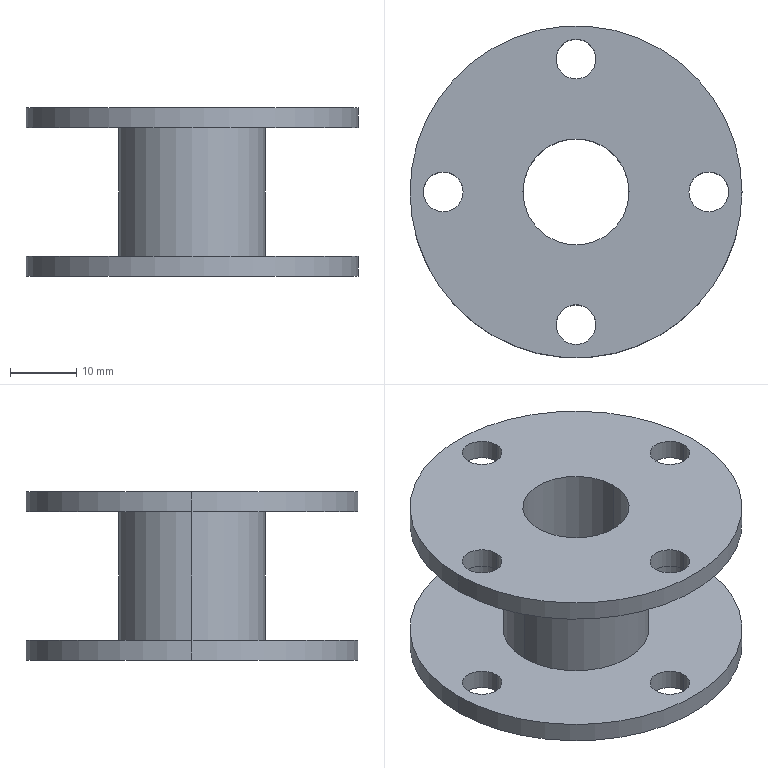Part | SolidWorks | features ExtruThin 1, ICE 1, MirrorPattern 1 | 1 solid | 28 faces | box 50 x 50 x 25.41 mm | volume 13372 mm3 | cylinder 24 | plane 4 | commonest cylinder face diameters 6 x16 50 x4 16 x2 22 x2
STEP:
#1=CARTESIAN_POINT('',(-23.,0.,-9.705));
#2=VERTEX_POINT('',#1);
#3=CARTESIAN_POINT('',(-17.,0.,-9.705));
#4=VERTEX_POINT('',#3);
#5=CARTESIAN_POINT('',(-20.,0.,-9.705));
#6=DIRECTION('',(0.,0.,1.));
#7=DIRECTION('',(1.,0.,0.));
#8=AXIS2_PLACEMENT_3D('',#5,#6,#7);
#9=CIRCLE('',#8,3.);
#10=EDGE_CURVE('',#2,#4,#9,.T.);
#11=ORIENTED_EDGE('',*,*,#10,.T.);
#12=CARTESIAN_POINT('',(-17.,0.,-12.705));
#13=VERTEX_POINT('',#12);
#14=CARTESIAN_POINT('',(-17.,0.,-9.705));
#15=DIRECTION('',(0.,0.,-1.));
#16=VECTOR('',#15,1000.);
#17=LINE('',#14,#16);
#18=EDGE_CURVE('',#4,#13,#17,.T.);
#19=ORIENTED_EDGE('',*,*,#18,.T.);
#20=CARTESIAN_POINT('',(-23.,0.,-12.705));
#21=VERTEX_POINT('',#20);
#22=CARTESIAN_POINT('',(-20.,0.,-12.705));
#23=DIRECTION('',(0.,0.,1.));
#24=DIRECTION('',(1.,0.,0.));
#25=AXIS2_PLACEMENT_3D('',#22,#23,#24);
#26=CIRCLE('',#25,3.);
#27=EDGE_CURVE('',#21,#13,#26,.T.);
#28=ORIENTED_EDGE('',*,*,#27,.F.);
#29=CARTESIAN_POINT('',(-23.,0.,-9.705));
#30=DIRECTION('',(0.,0.,-1.));
#31=VECTOR('',#30,1000.);
#32=LINE('',#29,#31);
#33=EDGE_CURVE('',#2,#21,#32,.T.);
#34=ORIENTED_EDGE('',*,*,#33,.F.);
#35=EDGE_LOOP('',(#11,#19,#28,#34));
#36=FACE_OUTER_BOUND('',#35,.T.);
#37=CARTESIAN_POINT('',(-20.,0.,-9.705));
#38=DIRECTION('',(0.,0.,-1.));
#39=DIRECTION('',(-1.,0.,0.));
#40=AXIS2_PLACEMENT_3D('',#37,#38,#39);
#41=CYLINDRICAL_SURFACE('',#40,3.);
#42=ADVANCED_FACE('',(#36),#41,.F.);
#43=CARTESIAN_POINT('',(-3.,-20.,-9.705));
#44=VERTEX_POINT('',#43);
#45=CARTESIAN_POINT('',(3.,-20.,-9.705));
#46=VERTEX_POINT('',#45);
#47=CARTESIAN_POINT('',(0.,-20.,-9.705));
#48=DIRECTION('',(0.,0.,1.));
#49=DIRECTION('',(1.,0.,0.));
#50=AXIS2_PLACEMENT_3D('',#47,#48,#49);
#51=CIRCLE('',#50,3.);
#52=EDGE_CURVE('',#44,#46,#51,.T.);
#53=ORIENTED_EDGE('',*,*,#52,.T.);
#54=CARTESIAN_POINT('',(3.,-20.,-12.705));
#55=VERTEX_POINT('',#54);
#56=CARTESIAN_POINT('',(3.,-20.,-9.705));
#57=DIRECTION('',(0.,0.,-1.));
#58=VECTOR('',#57,1000.);
#59=LINE('',#56,#58);
#60=EDGE_CURVE('',#46,#55,#59,.T.);
#61=ORIENTED_EDGE('',*,*,#60,.T.);
#62=CARTESIAN_POINT('',(-3.,-20.,-12.705));
#63=VERTEX_POINT('',#62);
#64=CARTESIAN_POINT('',(0.,-20.,-12.705));
#65=DIRECTION('',(0.,0.,1.));
#66=DIRECTION('',(1.,0.,0.));
#67=AXIS2_PLACEMENT_3D('',#64,#65,#66);
#68=CIRCLE('',#67,3.);
#69=EDGE_CURVE('',#63,#55,#68,.T.);
#70=ORIENTED_EDGE('',*,*,#69,.F.);
#71=CARTESIAN_POINT('',(-3.,-20.,-9.705));
#72=DIRECTION('',(0.,0.,-1.));
#73=VECTOR('',#72,1000.);
#74=LINE('',#71,#73);
#75=EDGE_CURVE('',#44,#63,#74,.T.);
#76=ORIENTED_EDGE('',*,*,#75,.F.);
#77=EDGE_LOOP('',(#53,#61,#70,#76));
#78=FACE_OUTER_BOUND('',#77,.T.);
#79=CARTESIAN_POINT('',(0.,-20.,-9.705));
#80=DIRECTION('',(0.,0.,-1.));
#81=DIRECTION('',(-1.,0.,0.));
#82=AXIS2_PLACEMENT_3D('',#79,#80,#81);
#83=CYLINDRICAL_SURFACE('',#82,3.);
#84=ADVANCED_FACE('',(#78),#83,.F.);
#85=CARTESIAN_POINT('',(17.,0.,-9.705));
#86=VERTEX_POINT('',#85);
#87=CARTESIAN_POINT('',(23.,0.,-9.705));
#88=VERTEX_POINT('',#87);
#89=CARTESIAN_POINT('',(20.,0.,-9.705));
#90=DIRECTION('',(0.,0.,1.));
#91=DIRECTION('',(1.,0.,0.));
#92=AXIS2_PLACEMENT_3D('',#89,#90,#91);
#93=CIRCLE('',#92,3.);
#94=EDGE_CURVE('',#86,#88,#93,.T.);
#95=ORIENTED_EDGE('',*,*,#94,.T.);
#96=CARTESIAN_POINT('',(23.,0.,-12.705));
#97=VERTEX_POINT('',#96);
#98=CARTESIAN_POINT('',(23.,0.,-9.705));
#99=DIRECTION('',(0.,0.,-1.));
#100=VECTOR('',#99,1000.);
#101=LINE('',#98,#100);
#102=EDGE_CURVE('',#88,#97,#101,.T.);
#103=ORIENTED_EDGE('',*,*,#102,.T.);
#104=CARTESIAN_POINT('',(17.,0.,-12.705));
#105=VERTEX_POINT('',#104);
#106=CARTESIAN_POINT('',(20.,0.,-12.705));
#107=DIRECTION('',(0.,0.,1.));
#108=DIRECTION('',(1.,0.,0.));
#109=AXIS2_PLACEMENT_3D('',#106,#107,#108);
#110=CIRCLE('',#109,3.);
#111=EDGE_CURVE('',#105,#97,#110,.T.);
#112=ORIENTED_EDGE('',*,*,#111,.F.);
#113=CARTESIAN_POINT('',(17.,0.,-9.705));
#114=DIRECTION('',(0.,0.,-1.));
#115=VECTOR('',#114,1000.);
#116=LINE('',#113,#115);
#117=EDGE_CURVE('',#86,#105,#116,.T.);
#118=ORIENTED_EDGE('',*,*,#117,.F.);
#119=EDGE_LOOP('',(#95,#103,#112,#118));
#120=FACE_OUTER_BOUND('',#119,.T.);
#121=CARTESIAN_POINT('',(20.,0.,-9.705));
#122=DIRECTION('',(0.,0.,-1.));
#123=DIRECTION('',(-1.,0.,0.));
#124=AXIS2_PLACEMENT_3D('',#121,#122,#123);
#125=CYLINDRICAL_SURFACE('',#124,3.);
#126=ADVANCED_FACE('',(#120),#125,.F.);
#127=CARTESIAN_POINT('',(-3.,20.,-9.705));
#128=VERTEX_POINT('',#127);
#129=CARTESIAN_POINT('',(3.,20.,-9.705));
#130=VERTEX_POINT('',#129);
#131=CARTESIAN_POINT('',(0.,20.,-9.705));
#132=DIRECTION('',(0.,0.,1.));
#133=DIRECTION('',(1.,0.,0.));
#134=AXIS2_PLACEMENT_3D('',#131,#132,#133);
#135=CIRCLE('',#134,3.);
#136=EDGE_CURVE('',#128,#130,#135,.T.);
#137=ORIENTED_EDGE('',*,*,#136,.T.);
#138=CARTESIAN_POINT('',(3.,20.,-12.705));
#139=VERTEX_POINT('',#138);
#140=CARTESIAN_POINT('',(3.,20.,-9.705));
#141=DIRECTION('',(0.,0.,-1.));
#142=VECTOR('',#141,1000.);
#143=LINE('',#140,#142);
#144=EDGE_CURVE('',#130,#139,#143,.T.);
#145=ORIENTED_EDGE('',*,*,#144,.T.);
#146=CARTESIAN_POINT('',(-3.,20.,-12.705));
#147=VERTEX_POINT('',#146);
#148=CARTESIAN_POINT('',(0.,20.,-12.705));
#149=DIRECTION('',(0.,0.,1.));
#150=DIRECTION('',(1.,0.,0.));
#151=AXIS2_PLACEMENT_3D('',#148,#149,#150);
#152=CIRCLE('',#151,3.);
#153=EDGE_CURVE('',#147,#139,#152,.T.);
#154=ORIENTED_EDGE('',*,*,#153,.F.);
#155=CARTESIAN_POINT('',(-3.,20.,-9.705));
#156=DIRECTION('',(0.,0.,-1.));
#157=VECTOR('',#156,1000.);
#158=LINE('',#155,#157);
#159=EDGE_CURVE('',#128,#147,#158,.T.);
#160=ORIENTED_EDGE('',*,*,#159,.F.);
#161=EDGE_LOOP('',(#137,#145,#154,#160));
#162=FACE_OUTER_BOUND('',#161,.T.);
#163=CARTESIAN_POINT('',(0.,20.,-9.705));
#164=DIRECTION('',(0.,0.,-1.));
#165=DIRECTION('',(-1.,0.,0.));
#166=AXIS2_PLACEMENT_3D('',#163,#164,#165);
#167=CYLINDRICAL_SURFACE('',#166,3.);
#168=ADVANCED_FACE('',(#162),#167,.F.);
#169=CARTESIAN_POINT('',(25.,0.,-9.705));
#170=VERTEX_POINT('',#169);
#171=CARTESIAN_POINT('',(-25.,0.,-9.705));
#172=VERTEX_POINT('',#171);
#173=CARTESIAN_POINT('',(0.,0.,-9.705));
#174=DIRECTION('',(0.,0.,1.));
#175=DIRECTION('',(1.,0.,0.));
#176=AXIS2_PLACEMENT_3D('',#173,#174,#175);
#177=CIRCLE('',#176,25.);
#178=EDGE_CURVE('',#170,#172,#177,.T.);
#179=ORIENTED_EDGE('',*,*,#178,.F.);
#180=CARTESIAN_POINT('',(25.,0.,-12.705));
#181=VERTEX_POINT('',#180);
#182=CARTESIAN_POINT('',(25.,0.,-9.705));
#183=DIRECTION('',(0.,0.,-1.));
#184=VECTOR('',#183,1000.);
#185=LINE('',#182,#184);
#186=EDGE_CURVE('',#170,#181,#185,.T.);
#187=ORIENTED_EDGE('',*,*,#186,.T.);
#188=CARTESIAN_POINT('',(-25.,0.,-12.705));
#189=VERTEX_POINT('',#188);
#190=CARTESIAN_POINT('',(0.,0.,-12.705));
#191=DIRECTION('',(0.,0.,1.));
#192=DIRECTION('',(1.,0.,0.));
#193=AXIS2_PLACEMENT_3D('',#190,#191,#192);
#194=CIRCLE('',#193,25.);
#195=EDGE_CURVE('',#181,#189,#194,.T.);
#196=ORIENTED_EDGE('',*,*,#195,.T.);
#197=CARTESIAN_POINT('',(-25.,0.,-9.705));
#198=DIRECTION('',(0.,0.,-1.));
#199=VECTOR('',#198,1000.);
#200=LINE('',#197,#199);
#201=EDGE_CURVE('',#172,#189,#200,.T.);
#202=ORIENTED_EDGE('',*,*,#201,.F.);
#203=EDGE_LOOP('',(#179,#187,#196,#202));
#204=FACE_OUTER_BOUND('',#203,.T.);
#205=CARTESIAN_POINT('',(0.,0.,-9.705));
#206=DIRECTION('',(0.,0.,-1.));
#207=DIRECTION('',(-1.,0.,0.));
#208=AXIS2_PLACEMENT_3D('',#205,#206,#207);
#209=CYLINDRICAL_SURFACE('',#208,25.);
#210=ADVANCED_FACE('',(#204),#209,.T.);
#211=CARTESIAN_POINT('',(-23.,0.,9.705));
#212=VERTEX_POINT('',#211);
#213=CARTESIAN_POINT('',(-17.,0.,9.705));
#214=VERTEX_POINT('',#213);
#215=CARTESIAN_POINT('',(-20.,0.,9.705));
#216=DIRECTION('',(0.,0.,1.));
#217=DIRECTION('',(1.,0.,0.));
#218=AXIS2_PLACEMENT_3D('',#215,#216,#217);
#219=CIRCLE('',#218,3.);
#220=EDGE_CURVE('',#212,#214,#219,.T.);
#221=ORIENTED_EDGE('',*,*,#220,.F.);
#222=CARTESIAN_POINT('',(-23.,0.,12.705));
#223=VERTEX_POINT('',#222);
#224=CARTESIAN_POINT('',(-23.,0.,9.705));
#225=DIRECTION('',(0.,0.,1.));
#226=VECTOR('',#225,1000.);
#227=LINE('',#224,#226);
#228=EDGE_CURVE('',#212,#223,#227,.T.);
#229=ORIENTED_EDGE('',*,*,#228,.T.);
#230=CARTESIAN_POINT('',(-17.,0.,12.705));
#231=VERTEX_POINT('',#230);
#232=CARTESIAN_POINT('',(-20.,0.,12.705));
#233=DIRECTION('',(0.,0.,1.));
#234=DIRECTION('',(1.,0.,0.));
#235=AXIS2_PLACEMENT_3D('',#232,#233,#234);
#236=CIRCLE('',#235,3.);
#237=EDGE_CURVE('',#223,#231,#236,.T.);
#238=ORIENTED_EDGE('',*,*,#237,.T.);
#239=CARTESIAN_POINT('',(-17.,0.,9.705));
#240=DIRECTION('',(0.,0.,1.));
#241=VECTOR('',#240,1000.);
#242=LINE('',#239,#241);
#243=EDGE_CURVE('',#214,#231,#242,.T.);
#244=ORIENTED_EDGE('',*,*,#243,.F.);
#245=EDGE_LOOP('',(#221,#229,#238,#244));
#246=FACE_OUTER_BOUND('',#245,.T.);
#247=CARTESIAN_POINT('',(-20.,0.,9.705));
#248=DIRECTION('',(0.,0.,1.));
#249=DIRECTION('',(1.,0.,0.));
#250=AXIS2_PLACEMENT_3D('',#247,#248,#249);
#251=CYLINDRICAL_SURFACE('',#250,3.);
#252=ADVANCED_FACE('',(#246),#251,.F.);
#253=CARTESIAN_POINT('',(-3.,-20.,9.705));
#254=VERTEX_POINT('',#253);
#255=CARTESIAN_POINT('',(3.,-20.,9.705));
#256=VERTEX_POINT('',#255);
#257=CARTESIAN_POINT('',(0.,-20.,9.705));
#258=DIRECTION('',(0.,0.,1.));
#259=DIRECTION('',(1.,0.,0.));
#260=AXIS2_PLACEMENT_3D('',#257,#258,#259);
#261=CIRCLE('',#260,3.);
#262=EDGE_CURVE('',#254,#256,#261,.T.);
#263=ORIENTED_EDGE('',*,*,#262,.F.);
#264=CARTESIAN_POINT('',(-3.,-20.,12.705));
#265=VERTEX_POINT('',#264);
#266=CARTESIAN_POINT('',(-3.,-20.,9.705));
#267=DIRECTION('',(0.,0.,1.));
#268=VECTOR('',#267,1000.);
#269=LINE('',#266,#268);
#270=EDGE_CURVE('',#254,#265,#269,.T.);
#271=ORIENTED_EDGE('',*,*,#270,.T.);
#272=CARTESIAN_POINT('',(3.,-20.,12.705));
#273=VERTEX_POINT('',#272);
#274=CARTESIAN_POINT('',(0.,-20.,12.705));
#275=DIRECTION('',(0.,0.,1.));
#276=DIRECTION('',(1.,0.,0.));
#277=AXIS2_PLACEMENT_3D('',#274,#275,#276);
#278=CIRCLE('',#277,3.);
#279=EDGE_CURVE('',#265,#273,#278,.T.);
#280=ORIENTED_EDGE('',*,*,#279,.T.);
#281=CARTESIAN_POINT('',(3.,-20.,9.705));
#282=DIRECTION('',(0.,0.,1.));
#283=VECTOR('',#282,1000.);
#284=LINE('',#281,#283);
#285=EDGE_CURVE('',#256,#273,#284,.T.);
#286=ORIENTED_EDGE('',*,*,#285,.F.);
#287=EDGE_LOOP('',(#263,#271,#280,#286));
#288=FACE_OUTER_BOUND('',#287,.T.);
#289=CARTESIAN_POINT('',(0.,-20.,9.705));
#290=DIRECTION('',(0.,0.,1.));
#291=DIRECTION('',(1.,0.,0.));
#292=AXIS2_PLACEMENT_3D('',#289,#290,#291);
#293=CYLINDRICAL_SURFACE('',#292,3.);
#294=ADVANCED_FACE('',(#288),#293,.F.);
#295=CARTESIAN_POINT('',(17.,0.,9.705));
#296=VERTEX_POINT('',#295);
#297=CARTESIAN_POINT('',(23.,0.,9.705));
#298=VERTEX_POINT('',#297);
#299=CARTESIAN_POINT('',(20.,0.,9.705));
#300=DIRECTION('',(0.,0.,1.));
#301=DIRECTION('',(1.,0.,0.));
#302=AXIS2_PLACEMENT_3D('',#299,#300,#301);
#303=CIRCLE('',#302,3.);
#304=EDGE_CURVE('',#296,#298,#303,.T.);
#305=ORIENTED_EDGE('',*,*,#304,.F.);
#306=CARTESIAN_POINT('',(17.,0.,12.705));
#307=VERTEX_POINT('',#306);
#308=CARTESIAN_POINT('',(17.,0.,9.705));
#309=DIRECTION('',(0.,0.,1.));
#310=VECTOR('',#309,1000.);
#311=LINE('',#308,#310);
#312=EDGE_CURVE('',#296,#307,#311,.T.);
#313=ORIENTED_EDGE('',*,*,#312,.T.);
#314=CARTESIAN_POINT('',(23.,0.,12.705));
#315=VERTEX_POINT('',#314);
#316=CARTESIAN_POINT('',(20.,0.,12.705));
#317=DIRECTION('',(0.,0.,1.));
#318=DIRECTION('',(1.,0.,0.));
#319=AXIS2_PLACEMENT_3D('',#316,#317,#318);
#320=CIRCLE('',#319,3.);
#321=EDGE_CURVE('',#307,#315,#320,.T.);
#322=ORIENTED_EDGE('',*,*,#321,.T.);
#323=CARTESIAN_POINT('',(23.,0.,9.705));
#324=DIRECTION('',(0.,0.,1.));
#325=VECTOR('',#324,1000.);
#326=LINE('',#323,#325);
#327=EDGE_CURVE('',#298,#315,#326,.T.);
#328=ORIENTED_EDGE('',*,*,#327,.F.);
#329=EDGE_LOOP('',(#305,#313,#322,#328));
#330=FACE_OUTER_BOUND('',#329,.T.);
#331=CARTESIAN_POINT('',(20.,0.,9.705));
#332=DIRECTION('',(0.,0.,1.));
#333=DIRECTION('',(1.,0.,0.));
#334=AXIS2_PLACEMENT_3D('',#331,#332,#333);
#335=CYLINDRICAL_SURFACE('',#334,3.);
#336=ADVANCED_FACE('',(#330),#335,.F.);
#337=CARTESIAN_POINT('',(-3.,20.,9.705));
#338=VERTEX_POINT('',#337);
#339=CARTESIAN_POINT('',(3.,20.,9.705));
#340=VERTEX_POINT('',#339);
#341=CARTESIAN_POINT('',(0.,20.,9.705));
#342=DIRECTION('',(0.,0.,1.));
#343=DIRECTION('',(1.,0.,0.));
#344=AXIS2_PLACEMENT_3D('',#341,#342,#343);
#345=CIRCLE('',#344,3.);
#346=EDGE_CURVE('',#338,#340,#345,.T.);
#347=ORIENTED_EDGE('',*,*,#346,.F.);
#348=CARTESIAN_POINT('',(-3.,20.,12.705));
#349=VERTEX_POINT('',#348);
#350=CARTESIAN_POINT('',(-3.,20.,9.705));
#351=DIRECTION('',(0.,0.,1.));
#352=VECTOR('',#351,1000.);
#353=LINE('',#350,#352);
#354=EDGE_CURVE('',#338,#349,#353,.T.);
#355=ORIENTED_EDGE('',*,*,#354,.T.);
#356=CARTESIAN_POINT('',(3.,20.,12.705));
#357=VERTEX_POINT('',#356);
#358=CARTESIAN_POINT('',(0.,20.,12.705));
#359=DIRECTION('',(0.,0.,1.));
#360=DIRECTION('',(1.,0.,0.));
#361=AXIS2_PLACEMENT_3D('',#358,#359,#360);
#362=CIRCLE('',#361,3.);
#363=EDGE_CURVE('',#349,#357,#362,.T.);
#364=ORIENTED_EDGE('',*,*,#363,.T.);
#365=CARTESIAN_POINT('',(3.,20.,9.705));
#366=DIRECTION('',(0.,0.,1.));
#367=VECTOR('',#366,1000.);
#368=LINE('',#365,#367);
#369=EDGE_CURVE('',#340,#357,#368,.T.);
#370=ORIENTED_EDGE('',*,*,#369,.F.);
#371=EDGE_LOOP('',(#347,#355,#364,#370));
#372=FACE_OUTER_BOUND('',#371,.T.);
#373=CARTESIAN_POINT('',(0.,20.,9.705));
#374=DIRECTION('',(0.,0.,1.));
#375=DIRECTION('',(1.,0.,0.));
#376=AXIS2_PLACEMENT_3D('',#373,#374,#375);
#377=CYLINDRICAL_SURFACE('',#376,3.);
#378=ADVANCED_FACE('',(#372),#377,.F.);
#379=CARTESIAN_POINT('',(25.,0.,9.705));
#380=VERTEX_POINT('',#379);
#381=CARTESIAN_POINT('',(-25.,0.,9.705));
#382=VERTEX_POINT('',#381);
#383=CARTESIAN_POINT('',(0.,0.,9.705));
#384=DIRECTION('',(0.,0.,1.));
#385=DIRECTION('',(1.,0.,0.));
#386=AXIS2_PLACEMENT_3D('',#383,#384,#385);
#387=CIRCLE('',#386,25.);
#388=EDGE_CURVE('',#380,#382,#387,.T.);
#389=ORIENTED_EDGE('',*,*,#388,.T.);
#390=CARTESIAN_POINT('',(-25.,0.,12.705));
#391=VERTEX_POINT('',#390);
#392=CARTESIAN_POINT('',(-25.,0.,9.705));
#393=DIRECTION('',(0.,0.,1.));
#394=VECTOR('',#393,1000.);
#395=LINE('',#392,#394);
#396=EDGE_CURVE('',#382,#391,#395,.T.);
#397=ORIENTED_EDGE('',*,*,#396,.T.);
#398=CARTESIAN_POINT('',(25.,0.,12.705));
#399=VERTEX_POINT('',#398);
#400=CARTESIAN_POINT('',(0.,0.,12.705));
#401=DIRECTION('',(0.,0.,1.));
#402=DIRECTION('',(1.,0.,0.));
#403=AXIS2_PLACEMENT_3D('',#400,#401,#402);
#404=CIRCLE('',#403,25.);
#405=EDGE_CURVE('',#399,#391,#404,.T.);
#406=ORIENTED_EDGE('',*,*,#405,.F.);
#407=CARTESIAN_POINT('',(25.,0.,9.705));
#408=DIRECTION('',(0.,0.,1.));
#409=VECTOR('',#408,1000.);
#410=LINE('',#407,#409);
#411=EDGE_CURVE('',#380,#399,#410,.T.);
#412=ORIENTED_EDGE('',*,*,#411,.F.);
#413=EDGE_LOOP('',(#389,#397,#406,#412));
#414=FACE_OUTER_BOUND('',#413,.T.);
#415=CARTESIAN_POINT('',(0.,0.,9.705));
#416=DIRECTION('',(0.,0.,1.));
#417=DIRECTION('',(1.,0.,0.));
#418=AXIS2_PLACEMENT_3D('',#415,#416,#417);
#419=CYLINDRICAL_SURFACE('',#418,25.);
#420=ADVANCED_FACE('',(#414),#419,.T.);
#421=CARTESIAN_POINT('',(-8.,0.,12.705));
#422=VERTEX_POINT('',#421);
#423=CARTESIAN_POINT('',(8.,0.,12.705));
#424=VERTEX_POINT('',#423);
#425=CARTESIAN_POINT('',(0.,0.,12.705));
#426=DIRECTION('',(0.,0.,1.));
#427=DIRECTION('',(1.,0.,0.));
#428=AXIS2_PLACEMENT_3D('',#425,#426,#427);
#429=CIRCLE('',#428,8.);
#430=EDGE_CURVE('',#422,#424,#429,.T.);
#431=ORIENTED_EDGE('',*,*,#430,.T.);
#432=CARTESIAN_POINT('',(8.,0.,-12.705));
#433=VERTEX_POINT('',#432);
#434=CARTESIAN_POINT('',(8.,0.,12.705));
#435=DIRECTION('',(0.,0.,-1.));
#436=VECTOR('',#435,1000.);
#437=LINE('',#434,#436);
#438=EDGE_CURVE('',#424,#433,#437,.T.);
#439=ORIENTED_EDGE('',*,*,#438,.T.);
#440=CARTESIAN_POINT('',(-8.,0.,-12.705));
#441=VERTEX_POINT('',#440);
#442=CARTESIAN_POINT('',(0.,0.,-12.705));
#443=DIRECTION('',(0.,0.,1.));
#444=DIRECTION('',(1.,0.,0.));
#445=AXIS2_PLACEMENT_3D('',#442,#443,#444);
#446=CIRCLE('',#445,8.);
#447=EDGE_CURVE('',#441,#433,#446,.T.);
#448=ORIENTED_EDGE('',*,*,#447,.F.);
#449=CARTESIAN_POINT('',(-8.,0.,12.705));
#450=DIRECTION('',(0.,0.,-1.));
#451=VECTOR('',#450,1000.);
#452=LINE('',#449,#451);
#453=EDGE_CURVE('',#422,#441,#452,.T.);
#454=ORIENTED_EDGE('',*,*,#453,.F.);
#455=EDGE_LOOP('',(#431,#439,#448,#454));
#456=FACE_OUTER_BOUND('',#455,.T.);
#457=CARTESIAN_POINT('',(0.,0.,12.705));
#458=DIRECTION('',(0.,0.,-1.));
#459=DIRECTION('',(-1.,0.,0.));
#460=AXIS2_PLACEMENT_3D('',#457,#458,#459);
#461=CYLINDRICAL_SURFACE('',#460,8.);
#462=ADVANCED_FACE('',(#456),#461,.F.);
#463=CARTESIAN_POINT('',(11.,0.,9.705));
#464=VERTEX_POINT('',#463);
#465=CARTESIAN_POINT('',(-11.,0.,9.705));
#466=VERTEX_POINT('',#465);
#467=CARTESIAN_POINT('',(0.,0.,9.705));
#468=DIRECTION('',(0.,0.,1.));
#469=DIRECTION('',(1.,0.,0.));
#470=AXIS2_PLACEMENT_3D('',#467,#468,#469);
#471=CIRCLE('',#470,11.);
#472=EDGE_CURVE('',#464,#466,#471,.T.);
#473=ORIENTED_EDGE('',*,*,#472,.F.);
#474=CARTESIAN_POINT('',(11.,0.,-9.705));
#475=VERTEX_POINT('',#474);
#476=CARTESIAN_POINT('',(11.,0.,12.705));
#477=DIRECTION('',(0.,0.,-1.));
#478=VECTOR('',#477,1000.);
#479=LINE('',#476,#478);
#480=EDGE_CURVE('',#464,#475,#479,.T.);
#481=ORIENTED_EDGE('',*,*,#480,.T.);
#482=CARTESIAN_POINT('',(-11.,0.,-9.705));
#483=VERTEX_POINT('',#482);
#484=CARTESIAN_POINT('',(0.,0.,-9.705));
#485=DIRECTION('',(0.,0.,-1.));
#486=DIRECTION('',(-1.,0.,0.));
#487=AXIS2_PLACEMENT_3D('',#484,#485,#486);
#488=CIRCLE('',#487,11.);
#489=EDGE_CURVE('',#483,#475,#488,.T.);
#490=ORIENTED_EDGE('',*,*,#489,.F.);
#491=CARTESIAN_POINT('',(-11.,0.,12.705));
#492=DIRECTION('',(0.,0.,-1.));
#493=VECTOR('',#492,1000.);
#494=LINE('',#491,#493);
#495=EDGE_CURVE('',#466,#483,#494,.T.);
#496=ORIENTED_EDGE('',*,*,#495,.F.);
#497=EDGE_LOOP('',(#473,#481,#490,#496));
#498=FACE_OUTER_BOUND('',#497,.T.);
#499=CARTESIAN_POINT('',(0.,0.,12.705));
#500=DIRECTION('',(0.,0.,-1.));
#501=DIRECTION('',(-1.,0.,0.));
#502=AXIS2_PLACEMENT_3D('',#499,#500,#501);
#503=CYLINDRICAL_SURFACE('',#502,11.);
#504=ADVANCED_FACE('',(#498),#503,.T.);
#505=ORIENTED_EDGE('',*,*,#480,.F.);
#506=CARTESIAN_POINT('',(0.,0.,9.705));
#507=DIRECTION('',(0.,0.,1.));
#508=DIRECTION('',(1.,0.,0.));
#509=AXIS2_PLACEMENT_3D('',#506,#507,#508);
#510=CIRCLE('',#509,11.);
#511=EDGE_CURVE('',#466,#464,#510,.T.);
#512=ORIENTED_EDGE('',*,*,#511,.F.);
#513=ORIENTED_EDGE('',*,*,#495,.T.);
#514=CARTESIAN_POINT('',(0.,0.,-9.705));
#515=DIRECTION('',(0.,0.,-1.));
#516=DIRECTION('',(-1.,0.,0.));
#517=AXIS2_PLACEMENT_3D('',#514,#515,#516);
#518=CIRCLE('',#517,11.);
#519=EDGE_CURVE('',#475,#483,#518,.T.);
#520=ORIENTED_EDGE('',*,*,#519,.F.);
#521=EDGE_LOOP('',(#505,#512,#513,#520));
#522=FACE_OUTER_BOUND('',#521,.T.);
#523=CARTESIAN_POINT('',(0.,0.,12.705));
#524=DIRECTION('',(0.,0.,-1.));
#525=DIRECTION('',(-1.,0.,0.));
#526=AXIS2_PLACEMENT_3D('',#523,#524,#525);
#527=CYLINDRICAL_SURFACE('',#526,11.);
#528=ADVANCED_FACE('',(#522),#527,.T.);
#529=ORIENTED_EDGE('',*,*,#430,.F.);
#530=CARTESIAN_POINT('',(0.,0.,12.705));
#531=DIRECTION('',(0.,0.,1.));
#532=DIRECTION('',(1.,0.,0.));
#533=AXIS2_PLACEMENT_3D('',#530,#531,#532);
#534=CIRCLE('',#533,8.);
#535=EDGE_CURVE('',#424,#422,#534,.T.);
#536=ORIENTED_EDGE('',*,*,#535,.F.);
#537=EDGE_LOOP('',(#529,#536));
#538=FACE_BOUND('',#537,.T.);
#539=ORIENTED_EDGE('',*,*,#405,.T.);
#540=CARTESIAN_POINT('',(0.,0.,12.705));
#541=DIRECTION('',(0.,0.,1.));
#542=DIRECTION('',(1.,0.,0.));
#543=AXIS2_PLACEMENT_3D('',#540,#541,#542);
#544=CIRCLE('',#543,25.);
#545=EDGE_CURVE('',#391,#399,#544,.T.);
#546=ORIENTED_EDGE('',*,*,#545,.T.);
#547=EDGE_LOOP('',(#539,#546));
#548=FACE_OUTER_BOUND('',#547,.T.);
#549=CARTESIAN_POINT('',(0.,20.,12.705));
#550=DIRECTION('',(0.,0.,1.));
#551=DIRECTION('',(1.,0.,0.));
#552=AXIS2_PLACEMENT_3D('',#549,#550,#551);
#553=CIRCLE('',#552,3.);
#554=EDGE_CURVE('',#357,#349,#553,.T.);
#555=ORIENTED_EDGE('',*,*,#554,.F.);
#556=ORIENTED_EDGE('',*,*,#363,.F.);
#557=EDGE_LOOP('',(#555,#556));
#558=FACE_BOUND('',#557,.T.);
#559=CARTESIAN_POINT('',(20.,0.,12.705));
#560=DIRECTION('',(0.,0.,1.));
#561=DIRECTION('',(1.,0.,0.));
#562=AXIS2_PLACEMENT_3D('',#559,#560,#561);
#563=CIRCLE('',#562,3.);
#564=EDGE_CURVE('',#315,#307,#563,.T.);
#565=ORIENTED_EDGE('',*,*,#564,.F.);
#566=ORIENTED_EDGE('',*,*,#321,.F.);
#567=EDGE_LOOP('',(#565,#566));
#568=FACE_BOUND('',#567,.T.);
#569=CARTESIAN_POINT('',(0.,-20.,12.705));
#570=DIRECTION('',(0.,0.,1.));
#571=DIRECTION('',(1.,0.,0.));
#572=AXIS2_PLACEMENT_3D('',#569,#570,#571);
#573=CIRCLE('',#572,3.);
#574=EDGE_CURVE('',#273,#265,#573,.T.);
#575=ORIENTED_EDGE('',*,*,#574,.F.);
#576=ORIENTED_EDGE('',*,*,#279,.F.);
#577=EDGE_LOOP('',(#575,#576));
#578=FACE_BOUND('',#577,.T.);
#579=CARTESIAN_POINT('',(-20.,0.,12.705));
#580=DIRECTION('',(0.,0.,1.));
#581=DIRECTION('',(1.,0.,0.));
#582=AXIS2_PLACEMENT_3D('',#579,#580,#581);
#583=CIRCLE('',#582,3.);
#584=EDGE_CURVE('',#231,#223,#583,.T.);
#585=ORIENTED_EDGE('',*,*,#584,.F.);
#586=ORIENTED_EDGE('',*,*,#237,.F.);
#587=EDGE_LOOP('',(#585,#586));
#588=FACE_BOUND('',#587,.T.);
#589=CARTESIAN_POINT('',(0.,0.,12.705));
#590=DIRECTION('',(0.,0.,1.));
#591=DIRECTION('',(1.,0.,0.));
#592=AXIS2_PLACEMENT_3D('',#589,#590,#591);
#593=PLANE('',#592);
#594=ADVANCED_FACE('',(#538,#548,#558,#568,#578,#588),#593,.T.);
#595=ORIENTED_EDGE('',*,*,#447,.T.);
#596=CARTESIAN_POINT('',(0.,0.,-12.705));
#597=DIRECTION('',(0.,0.,1.));
#598=DIRECTION('',(1.,0.,0.));
#599=AXIS2_PLACEMENT_3D('',#596,#597,#598);
#600=CIRCLE('',#599,8.);
#601=EDGE_CURVE('',#433,#441,#600,.T.);
#602=ORIENTED_EDGE('',*,*,#601,.T.);
#603=EDGE_LOOP('',(#595,#602));
#604=FACE_BOUND('',#603,.T.);
#605=ORIENTED_EDGE('',*,*,#27,.T.);
#606=CARTESIAN_POINT('',(-20.,0.,-12.705));
#607=DIRECTION('',(0.,0.,1.));
#608=DIRECTION('',(1.,0.,0.));
#609=AXIS2_PLACEMENT_3D('',#606,#607,#608);
#610=CIRCLE('',#609,3.);
#611=EDGE_CURVE('',#13,#21,#610,.T.);
#612=ORIENTED_EDGE('',*,*,#611,.T.);
#613=EDGE_LOOP('',(#605,#612));
#614=FACE_BOUND('',#613,.T.);
#615=ORIENTED_EDGE('',*,*,#111,.T.);
#616=CARTESIAN_POINT('',(20.,0.,-12.705));
#617=DIRECTION('',(0.,0.,1.));
#618=DIRECTION('',(1.,0.,0.));
#619=AXIS2_PLACEMENT_3D('',#616,#617,#618);
#620=CIRCLE('',#619,3.);
#621=EDGE_CURVE('',#97,#105,#620,.T.);
#622=ORIENTED_EDGE('',*,*,#621,.T.);
#623=EDGE_LOOP('',(#615,#622));
#624=FACE_BOUND('',#623,.T.);
#625=CARTESIAN_POINT('',(0.,0.,-12.705));
#626=DIRECTION('',(0.,0.,1.));
#627=DIRECTION('',(1.,0.,0.));
#628=AXIS2_PLACEMENT_3D('',#625,#626,#627);
#629=CIRCLE('',#628,25.);
#630=EDGE_CURVE('',#189,#181,#629,.T.);
#631=ORIENTED_EDGE('',*,*,#630,.F.);
#632=ORIENTED_EDGE('',*,*,#195,.F.);
#633=EDGE_LOOP('',(#631,#632));
#634=FACE_OUTER_BOUND('',#633,.T.);
#635=ORIENTED_EDGE('',*,*,#153,.T.);
#636=CARTESIAN_POINT('',(0.,20.,-12.705));
#637=DIRECTION('',(0.,0.,1.));
#638=DIRECTION('',(1.,0.,0.));
#639=AXIS2_PLACEMENT_3D('',#636,#637,#638);
#640=CIRCLE('',#639,3.);
#641=EDGE_CURVE('',#139,#147,#640,.T.);
#642=ORIENTED_EDGE('',*,*,#641,.T.);
#643=EDGE_LOOP('',(#635,#642));
#644=FACE_BOUND('',#643,.T.);
#645=ORIENTED_EDGE('',*,*,#69,.T.);
#646=CARTESIAN_POINT('',(0.,-20.,-12.705));
#647=DIRECTION('',(0.,0.,1.));
#648=DIRECTION('',(1.,0.,0.));
#649=AXIS2_PLACEMENT_3D('',#646,#647,#648);
#650=CIRCLE('',#649,3.);
#651=EDGE_CURVE('',#55,#63,#650,.T.);
#652=ORIENTED_EDGE('',*,*,#651,.T.);
#653=EDGE_LOOP('',(#645,#652));
#654=FACE_BOUND('',#653,.T.);
#655=CARTESIAN_POINT('',(0.,0.,-12.705));
#656=DIRECTION('',(0.,0.,1.));
#657=DIRECTION('',(1.,0.,0.));
#658=AXIS2_PLACEMENT_3D('',#655,#656,#657);
#659=PLANE('',#658);
#660=ADVANCED_FACE('',(#604,#614,#624,#634,#644,#654),#659,.F.);
#661=ORIENTED_EDGE('',*,*,#438,.F.);
#662=ORIENTED_EDGE('',*,*,#535,.T.);
#663=ORIENTED_EDGE('',*,*,#453,.T.);
#664=ORIENTED_EDGE('',*,*,#601,.F.);
#665=EDGE_LOOP('',(#661,#662,#663,#664));
#666=FACE_OUTER_BOUND('',#665,.T.);
#667=CARTESIAN_POINT('',(0.,0.,12.705));
#668=DIRECTION('',(0.,0.,-1.));
#669=DIRECTION('',(-1.,0.,0.));
#670=AXIS2_PLACEMENT_3D('',#667,#668,#669);
#671=CYLINDRICAL_SURFACE('',#670,8.);
#672=ADVANCED_FACE('',(#666),#671,.F.);
#673=ORIENTED_EDGE('',*,*,#388,.F.);
#674=CARTESIAN_POINT('',(0.,0.,9.705));
#675=DIRECTION('',(0.,0.,1.));
#676=DIRECTION('',(1.,0.,0.));
#677=AXIS2_PLACEMENT_3D('',#674,#675,#676);
#678=CIRCLE('',#677,25.);
#679=EDGE_CURVE('',#382,#380,#678,.T.);
#680=ORIENTED_EDGE('',*,*,#679,.F.);
#681=EDGE_LOOP('',(#673,#680));
#682=FACE_OUTER_BOUND('',#681,.T.);
#683=CARTESIAN_POINT('',(0.,20.,9.705));
#684=DIRECTION('',(0.,0.,1.));
#685=DIRECTION('',(1.,0.,0.));
#686=AXIS2_PLACEMENT_3D('',#683,#684,#685);
#687=CIRCLE('',#686,3.);
#688=EDGE_CURVE('',#340,#338,#687,.T.);
#689=ORIENTED_EDGE('',*,*,#688,.T.);
#690=ORIENTED_EDGE('',*,*,#346,.T.);
#691=EDGE_LOOP('',(#689,#690));
#692=FACE_BOUND('',#691,.T.);
#693=CARTESIAN_POINT('',(20.,0.,9.705));
#694=DIRECTION('',(0.,0.,1.));
#695=DIRECTION('',(1.,0.,0.));
#696=AXIS2_PLACEMENT_3D('',#693,#694,#695);
#697=CIRCLE('',#696,3.);
#698=EDGE_CURVE('',#298,#296,#697,.T.);
#699=ORIENTED_EDGE('',*,*,#698,.T.);
#700=ORIENTED_EDGE('',*,*,#304,.T.);
#701=EDGE_LOOP('',(#699,#700));
#702=FACE_BOUND('',#701,.T.);
#703=CARTESIAN_POINT('',(0.,-20.,9.705));
#704=DIRECTION('',(0.,0.,1.));
#705=DIRECTION('',(1.,0.,0.));
#706=AXIS2_PLACEMENT_3D('',#703,#704,#705);
#707=CIRCLE('',#706,3.);
#708=EDGE_CURVE('',#256,#254,#707,.T.);
#709=ORIENTED_EDGE('',*,*,#708,.T.);
#710=ORIENTED_EDGE('',*,*,#262,.T.);
#711=EDGE_LOOP('',(#709,#710));
#712=FACE_BOUND('',#711,.T.);
#713=CARTESIAN_POINT('',(-20.,0.,9.705));
#714=DIRECTION('',(0.,0.,1.));
#715=DIRECTION('',(1.,0.,0.));
#716=AXIS2_PLACEMENT_3D('',#713,#714,#715);
#717=CIRCLE('',#716,3.);
#718=EDGE_CURVE('',#214,#212,#717,.T.);
#719=ORIENTED_EDGE('',*,*,#718,.T.);
#720=ORIENTED_EDGE('',*,*,#220,.T.);
#721=EDGE_LOOP('',(#719,#720));
#722=FACE_BOUND('',#721,.T.);
#723=ORIENTED_EDGE('',*,*,#511,.T.);
#724=ORIENTED_EDGE('',*,*,#472,.T.);
#725=EDGE_LOOP('',(#723,#724));
#726=FACE_BOUND('',#725,.T.);
#727=CARTESIAN_POINT('',(0.,0.,9.705));
#728=DIRECTION('',(0.,0.,1.));
#729=DIRECTION('',(1.,0.,0.));
#730=AXIS2_PLACEMENT_3D('',#727,#728,#729);
#731=PLANE('',#730);
#732=ADVANCED_FACE('',(#682,#692,#702,#712,#722,#726),#731,.F.);
#733=ORIENTED_EDGE('',*,*,#396,.F.);
#734=ORIENTED_EDGE('',*,*,#679,.T.);
#735=ORIENTED_EDGE('',*,*,#411,.T.);
#736=ORIENTED_EDGE('',*,*,#545,.F.);
#737=EDGE_LOOP('',(#733,#734,#735,#736));
#738=FACE_OUTER_BOUND('',#737,.T.);
#739=CARTESIAN_POINT('',(0.,0.,9.705));
#740=DIRECTION('',(0.,0.,1.));
#741=DIRECTION('',(1.,0.,0.));
#742=AXIS2_PLACEMENT_3D('',#739,#740,#741);
#743=CYLINDRICAL_SURFACE('',#742,25.);
#744=ADVANCED_FACE('',(#738),#743,.T.);
#745=ORIENTED_EDGE('',*,*,#354,.F.);
#746=ORIENTED_EDGE('',*,*,#688,.F.);
#747=ORIENTED_EDGE('',*,*,#369,.T.);
#748=ORIENTED_EDGE('',*,*,#554,.T.);
#749=EDGE_LOOP('',(#745,#746,#747,#748));
#750=FACE_OUTER_BOUND('',#749,.T.);
#751=CARTESIAN_POINT('',(0.,20.,9.705));
#752=DIRECTION('',(0.,0.,1.));
#753=DIRECTION('',(1.,0.,0.));
#754=AXIS2_PLACEMENT_3D('',#751,#752,#753);
#755=CYLINDRICAL_SURFACE('',#754,3.);
#756=ADVANCED_FACE('',(#750),#755,.F.);
#757=ORIENTED_EDGE('',*,*,#312,.F.);
#758=ORIENTED_EDGE('',*,*,#698,.F.);
#759=ORIENTED_EDGE('',*,*,#327,.T.);
#760=ORIENTED_EDGE('',*,*,#564,.T.);
#761=EDGE_LOOP('',(#757,#758,#759,#760));
#762=FACE_OUTER_BOUND('',#761,.T.);
#763=CARTESIAN_POINT('',(20.,0.,9.705));
#764=DIRECTION('',(0.,0.,1.));
#765=DIRECTION('',(1.,0.,0.));
#766=AXIS2_PLACEMENT_3D('',#763,#764,#765);
#767=CYLINDRICAL_SURFACE('',#766,3.);
#768=ADVANCED_FACE('',(#762),#767,.F.);
#769=ORIENTED_EDGE('',*,*,#270,.F.);
#770=ORIENTED_EDGE('',*,*,#708,.F.);
#771=ORIENTED_EDGE('',*,*,#285,.T.);
#772=ORIENTED_EDGE('',*,*,#574,.T.);
#773=EDGE_LOOP('',(#769,#770,#771,#772));
#774=FACE_OUTER_BOUND('',#773,.T.);
#775=CARTESIAN_POINT('',(0.,-20.,9.705));
#776=DIRECTION('',(0.,0.,1.));
#777=DIRECTION('',(1.,0.,0.));
#778=AXIS2_PLACEMENT_3D('',#775,#776,#777);
#779=CYLINDRICAL_SURFACE('',#778,3.);
#780=ADVANCED_FACE('',(#774),#779,.F.);
#781=ORIENTED_EDGE('',*,*,#228,.F.);
#782=ORIENTED_EDGE('',*,*,#718,.F.);
#783=ORIENTED_EDGE('',*,*,#243,.T.);
#784=ORIENTED_EDGE('',*,*,#584,.T.);
#785=EDGE_LOOP('',(#781,#782,#783,#784));
#786=FACE_OUTER_BOUND('',#785,.T.);
#787=CARTESIAN_POINT('',(-20.,0.,9.705));
#788=DIRECTION('',(0.,0.,1.));
#789=DIRECTION('',(1.,0.,0.));
#790=AXIS2_PLACEMENT_3D('',#787,#788,#789);
#791=CYLINDRICAL_SURFACE('',#790,3.);
#792=ADVANCED_FACE('',(#786),#791,.F.);
#793=ORIENTED_EDGE('',*,*,#10,.F.);
#794=CARTESIAN_POINT('',(-20.,0.,-9.705));
#795=DIRECTION('',(0.,0.,1.));
#796=DIRECTION('',(1.,0.,0.));
#797=AXIS2_PLACEMENT_3D('',#794,#795,#796);
#798=CIRCLE('',#797,3.);
#799=EDGE_CURVE('',#4,#2,#798,.T.);
#800=ORIENTED_EDGE('',*,*,#799,.F.);
#801=EDGE_LOOP('',(#793,#800));
#802=FACE_BOUND('',#801,.T.);
#803=ORIENTED_EDGE('',*,*,#52,.F.);
#804=CARTESIAN_POINT('',(0.,-20.,-9.705));
#805=DIRECTION('',(0.,0.,1.));
#806=DIRECTION('',(1.,0.,0.));
#807=AXIS2_PLACEMENT_3D('',#804,#805,#806);
#808=CIRCLE('',#807,3.);
#809=EDGE_CURVE('',#46,#44,#808,.T.);
#810=ORIENTED_EDGE('',*,*,#809,.F.);
#811=EDGE_LOOP('',(#803,#810));
#812=FACE_BOUND('',#811,.T.);
#813=ORIENTED_EDGE('',*,*,#94,.F.);
#814=CARTESIAN_POINT('',(20.,0.,-9.705));
#815=DIRECTION('',(0.,0.,1.));
#816=DIRECTION('',(1.,0.,0.));
#817=AXIS2_PLACEMENT_3D('',#814,#815,#816);
#818=CIRCLE('',#817,3.);
#819=EDGE_CURVE('',#88,#86,#818,.T.);
#820=ORIENTED_EDGE('',*,*,#819,.F.);
#821=EDGE_LOOP('',(#813,#820));
#822=FACE_BOUND('',#821,.T.);
#823=ORIENTED_EDGE('',*,*,#136,.F.);
#824=CARTESIAN_POINT('',(0.,20.,-9.705));
#825=DIRECTION('',(0.,0.,1.));
#826=DIRECTION('',(1.,0.,0.));
#827=AXIS2_PLACEMENT_3D('',#824,#825,#826);
#828=CIRCLE('',#827,3.);
#829=EDGE_CURVE('',#130,#128,#828,.T.);
#830=ORIENTED_EDGE('',*,*,#829,.F.);
#831=EDGE_LOOP('',(#823,#830));
#832=FACE_BOUND('',#831,.T.);
#833=CARTESIAN_POINT('',(0.,0.,-9.705));
#834=DIRECTION('',(0.,0.,1.));
#835=DIRECTION('',(1.,0.,0.));
#836=AXIS2_PLACEMENT_3D('',#833,#834,#835);
#837=CIRCLE('',#836,25.);
#838=EDGE_CURVE('',#172,#170,#837,.T.);
#839=ORIENTED_EDGE('',*,*,#838,.T.);
#840=ORIENTED_EDGE('',*,*,#178,.T.);
#841=EDGE_LOOP('',(#839,#840));
#842=FACE_OUTER_BOUND('',#841,.T.);
#843=ORIENTED_EDGE('',*,*,#489,.T.);
#844=ORIENTED_EDGE('',*,*,#519,.T.);
#845=EDGE_LOOP('',(#843,#844));
#846=FACE_BOUND('',#845,.T.);
#847=CARTESIAN_POINT('',(0.,0.,-9.705));
#848=DIRECTION('',(0.,0.,-1.));
#849=DIRECTION('',(1.,0.,0.));
#850=AXIS2_PLACEMENT_3D('',#847,#848,#849);
#851=PLANE('',#850);
#852=ADVANCED_FACE('',(#802,#812,#822,#832,#842,#846),#851,.F.);
#853=ORIENTED_EDGE('',*,*,#186,.F.);
#854=ORIENTED_EDGE('',*,*,#838,.F.);
#855=ORIENTED_EDGE('',*,*,#201,.T.);
#856=ORIENTED_EDGE('',*,*,#630,.T.);
#857=EDGE_LOOP('',(#853,#854,#855,#856));
#858=FACE_OUTER_BOUND('',#857,.T.);
#859=CARTESIAN_POINT('',(0.,0.,-9.705));
#860=DIRECTION('',(0.,0.,-1.));
#861=DIRECTION('',(-1.,0.,0.));
#862=AXIS2_PLACEMENT_3D('',#859,#860,#861);
#863=CYLINDRICAL_SURFACE('',#862,25.);
#864=ADVANCED_FACE('',(#858),#863,.T.);
#865=ORIENTED_EDGE('',*,*,#144,.F.);
#866=ORIENTED_EDGE('',*,*,#829,.T.);
#867=ORIENTED_EDGE('',*,*,#159,.T.);
#868=ORIENTED_EDGE('',*,*,#641,.F.);
#869=EDGE_LOOP('',(#865,#866,#867,#868));
#870=FACE_OUTER_BOUND('',#869,.T.);
#871=CARTESIAN_POINT('',(0.,20.,-9.705));
#872=DIRECTION('',(0.,0.,-1.));
#873=DIRECTION('',(-1.,0.,0.));
#874=AXIS2_PLACEMENT_3D('',#871,#872,#873);
#875=CYLINDRICAL_SURFACE('',#874,3.);
#876=ADVANCED_FACE('',(#870),#875,.F.);
#877=ORIENTED_EDGE('',*,*,#102,.F.);
#878=ORIENTED_EDGE('',*,*,#819,.T.);
#879=ORIENTED_EDGE('',*,*,#117,.T.);
#880=ORIENTED_EDGE('',*,*,#621,.F.);
#881=EDGE_LOOP('',(#877,#878,#879,#880));
#882=FACE_OUTER_BOUND('',#881,.T.);
#883=CARTESIAN_POINT('',(20.,0.,-9.705));
#884=DIRECTION('',(0.,0.,-1.));
#885=DIRECTION('',(-1.,0.,0.));
#886=AXIS2_PLACEMENT_3D('',#883,#884,#885);
#887=CYLINDRICAL_SURFACE('',#886,3.);
#888=ADVANCED_FACE('',(#882),#887,.F.);
#889=ORIENTED_EDGE('',*,*,#60,.F.);
#890=ORIENTED_EDGE('',*,*,#809,.T.);
#891=ORIENTED_EDGE('',*,*,#75,.T.);
#892=ORIENTED_EDGE('',*,*,#651,.F.);
#893=EDGE_LOOP('',(#889,#890,#891,#892));
#894=FACE_OUTER_BOUND('',#893,.T.);
#895=CARTESIAN_POINT('',(0.,-20.,-9.705));
#896=DIRECTION('',(0.,0.,-1.));
#897=DIRECTION('',(-1.,0.,0.));
#898=AXIS2_PLACEMENT_3D('',#895,#896,#897);
#899=CYLINDRICAL_SURFACE('',#898,3.);
#900=ADVANCED_FACE('',(#894),#899,.F.);
#901=ORIENTED_EDGE('',*,*,#18,.F.);
#902=ORIENTED_EDGE('',*,*,#799,.T.);
#903=ORIENTED_EDGE('',*,*,#33,.T.);
#904=ORIENTED_EDGE('',*,*,#611,.F.);
#905=EDGE_LOOP('',(#901,#902,#903,#904));
#906=FACE_OUTER_BOUND('',#905,.T.);
#907=CARTESIAN_POINT('',(-20.,0.,-9.705));
#908=DIRECTION('',(0.,0.,-1.));
#909=DIRECTION('',(-1.,0.,0.));
#910=AXIS2_PLACEMENT_3D('',#907,#908,#909);
#911=CYLINDRICAL_SURFACE('',#910,3.);
#912=ADVANCED_FACE('',(#906),#911,.F.);
#913=CLOSED_SHELL('',(#42,#84,#126,#168,#210,#252,#294,#336,#378,#420,#462,#504,#528,#594,#660,#672,#732,#744,#756,#768,#780,#792,#852,#864,#876,#888,#900,#912));
#914=MANIFOLD_SOLID_BREP('',#913);
#915=CARTESIAN_POINT('',(0.,0.,0.));
#916=DIRECTION('',(0.,0.,1.));
#917=DIRECTION('',(1.,0.,0.));
#918=AXIS2_PLACEMENT_3D('',#915,#916,#917);
#919=(LENGTH_UNIT()NAMED_UNIT(*)SI_UNIT(.MILLI.,.METRE.));
#920=UNCERTAINTY_MEASURE_WITH_UNIT(LENGTH_MEASURE(0.00001),#919,'','');
#921=(NAMED_UNIT(*)PLANE_ANGLE_UNIT()SI_UNIT($,.RADIAN.));
#922=(NAMED_UNIT(*)SI_UNIT($,.STERADIAN.)SOLID_ANGLE_UNIT());
#923=(GEOMETRIC_REPRESENTATION_CONTEXT(3)GLOBAL_UNCERTAINTY_ASSIGNED_CONTEXT((#920))GLOBAL_UNIT_ASSIGNED_CONTEXT((#919,#921,#922))REPRESENTATION_CONTEXT('',''));
#924=ADVANCED_BREP_SHAPE_REPRESENTATION('',(#914,#918),#923);